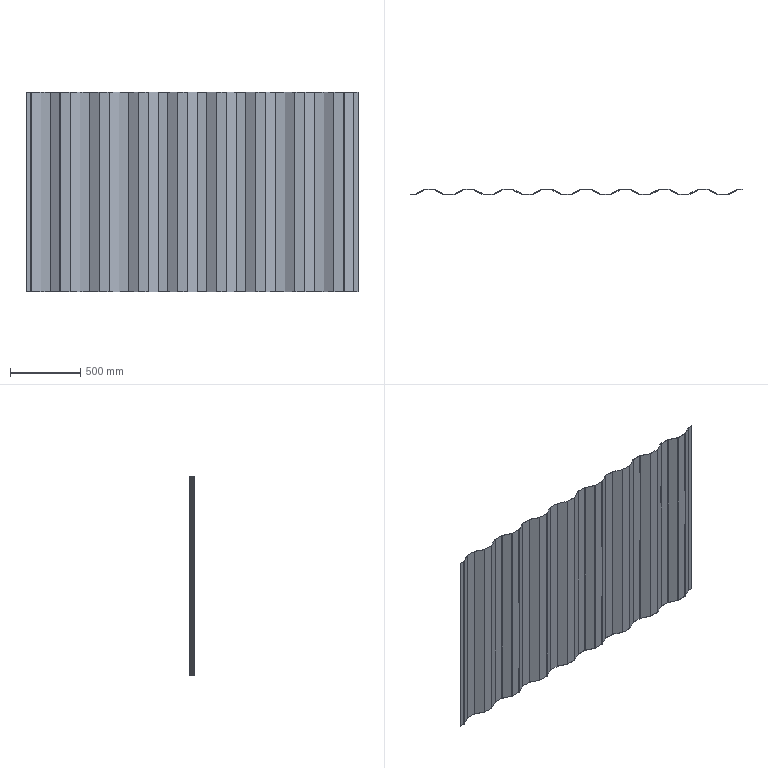Part | STEP file | 750038164 | 1 solid | 142 faces | box 2360 x 36 x 1416 mm | volume 7069165 mm3 | plane 74 | cylinder 68 | commonest cylinder face diameters 6 x34 10 x34